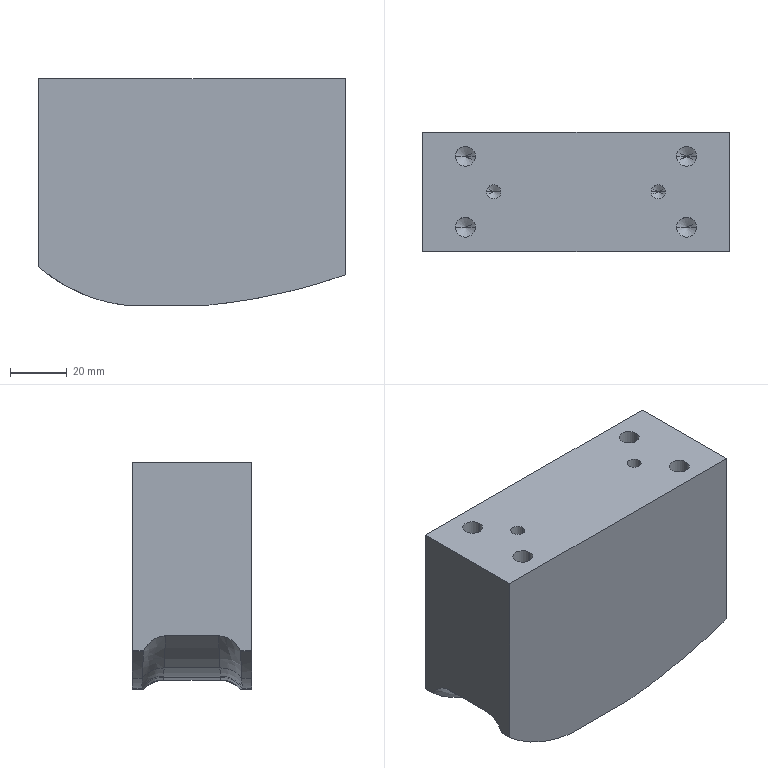Part | 1 solid | 99 faces | box 108 x 42 x 80.096 mm | volume 331401 mm3 | cylinder 42 | spline 30 | plane 15 | cone 12 | commonest cylinder face diameters 7 x8 18.81 x6 5 x4 111.103 x2 118.512 x2 203.901 x2